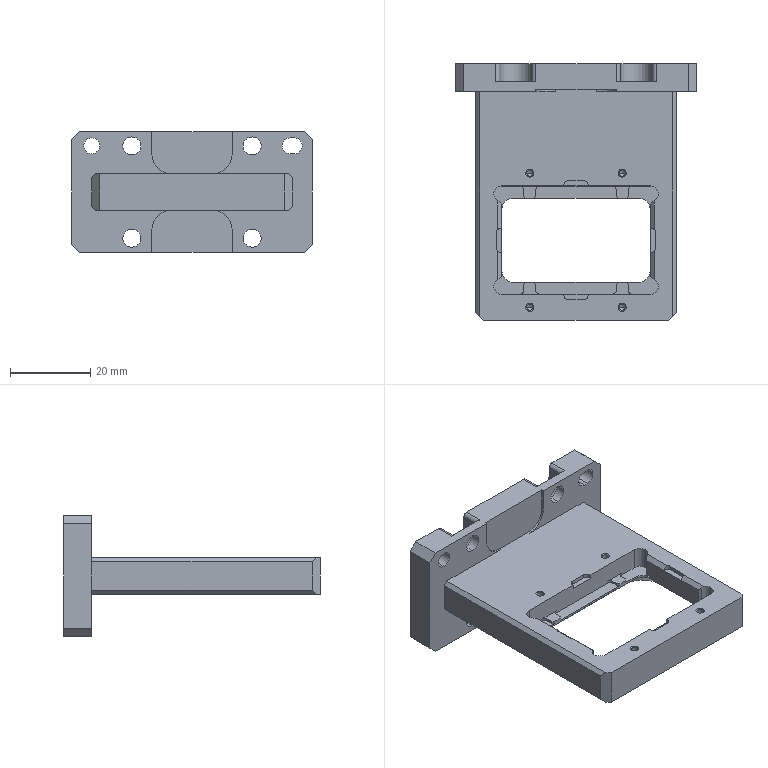NC program | NX | posted with a generic post | part box 60 x 64 x 30 mm
Lines 593 to 2202 of 2202, first 1347 of 1600 lines:
(HOLE_MILLING_COPY , TOOL : D3)
N1184 T03 M6
N1186 G54
N1188 G17 G0 G90 X-25. Y-11.48 B0. C0. S9500 M3
N1190 G43 Z30. H3
N1192 Z0.5
N1194 G94 G3 X-24.8 Y-11.68 R0.2 F1250.
N1196 X-24.6 Y-11.48 R0.2
N1198 X-24.6 Y-11.48 Z0.3 I-0.4 J0.
N1200 X-24.6 Y-11.48 Z0.1 I-0.4 J0.
N1202 X-24.6 Y-11.48 Z-0.1 I-0.4 J0.
N1204 X-24.6 Y-11.48 Z-0.3 I-0.4 J0.
N1206 X-24.6 Y-11.48 Z-0.5 I-0.4 J0.
N1208 X-24.6 Y-11.48 Z-0.7 I-0.4 J0.
N1210 X-24.6 Y-11.48 Z-0.9 I-0.4 J0.
N1212 X-24.6 Y-11.48 Z-1.1 I-0.4 J0.
N1214 X-24.6 Y-11.48 Z-1.3 I-0.4 J0.
N1216 X-24.6 Y-11.48 Z-1.5 I-0.4 J0.
N1218 X-24.6 Y-11.48 Z-1.7 I-0.4 J0.
N1220 X-24.6 Y-11.48 Z-1.9 I-0.4 J0.
N1222 X-24.6 Y-11.48 Z-2.1 I-0.4 J0.
N1224 X-24.6 Y-11.48 Z-2.3 I-0.4 J0.
N1226 X-24.6 Y-11.48 Z-2.5 I-0.4 J0.
N1228 X-24.6 Y-11.48 Z-2.7 I-0.4 J0.
N1230 X-24.6 Y-11.48 Z-2.9 I-0.4 J0.
N1232 X-24.6 Y-11.48 Z-3.1 I-0.4 J0.
N1234 X-24.6 Y-11.48 Z-3.3 I-0.4 J0.
N1236 X-24.6 Y-11.48 Z-3.5 I-0.4 J0.
N1238 X-24.6 Y-11.48 Z-3.7 I-0.4 J0.
N1240 X-24.6 Y-11.48 Z-3.9 I-0.4 J0.
N1242 X-24.6 Y-11.48 Z-4.1 I-0.4 J0.
N1244 X-24.6 Y-11.48 Z-4.3 I-0.4 J0.
N1246 X-24.6 Y-11.48 Z-4.5 I-0.4 J0.
N1248 X-24.6 Y-11.48 Z-4.7 I-0.4 J0.
N1250 X-24.6 Y-11.48 Z-4.9 I-0.4 J0.
N1252 X-24.6 Y-11.48 Z-5.1 I-0.4 J0.
N1254 X-24.6 Y-11.48 Z-5.3 I-0.4 J0.
N1256 X-24.6 Y-11.48 Z-5.5 I-0.4 J0.
N1258 X-24.6 Y-11.48 Z-5.7 I-0.4 J0.
N1260 X-24.6 Y-11.48 Z-5.9 I-0.4 J0.
N1262 X-24.6 Y-11.48 Z-6.1 I-0.4 J0.
N1264 X-24.6 Y-11.48 Z-6.3 I-0.4 J0.
N1266 X-24.6 Y-11.48 Z-6.5 I-0.4 J0.
N1268 X-24.6 Y-11.48 Z-6.7 I-0.4 J0.
N1270 X-24.6 Y-11.48 Z-6.9 I-0.4 J0.
N1272 X-25.4 Y-11.48 Z-7. I-0.4 J0.
N1274 X-25. Y-11.88 R0.4
N1276 X-25.4 Y-11.48 R-0.4
N1278 X-25.2 Y-11.68 R0.2
N1280 X-25. Y-11.48 R0.2
N1282 G0 Z30.
(ZLEVEL_PROFILE_1_1 , TOOL : D3)
N1284 X24.883 Y-11.88
N1286 Z1.
N1288 G1 X25.59 Z0.963 F1000.
N1290 X25.752 Y-11.803 Z0.954
N1292 X25.867 Y-11.664 Z0.944
N1294 X25.91 Y-11.478 Z0.934
N1296 X25.864 Y-11.292 Z0.924
N1298 X25.749 Y-11.154 Z0.915
N1300 X25.59 Y-11.08 Z0.905
N1302 X24.41 Z0.844
N1304 X24.314 Y-11.114 Z0.838
N1306 X24.176 Y-11.229 Z0.829
N1308 X24.1 Y-11.391 Z0.819
N1310 Y-11.57 Z0.81
N1312 X24.177 Y-11.732 Z0.801
N1314 X24.316 Y-11.846 Z0.791
N1316 X24.41 Y-11.88 Z0.786
N1318 X25.59 Z0.724
N1320 X25.752 Y-11.803 Z0.715
N1322 X25.867 Y-11.664 Z0.705
N1324 X25.91 Y-11.478 Z0.695
N1326 X25.864 Y-11.292 Z0.685
N1328 X25.749 Y-11.154 Z0.676
N1330 X25.59 Y-11.08 Z0.667
N1332 X24.41 Z0.605
N1334 X24.314 Y-11.114 Z0.599
N1336 X24.176 Y-11.229 Z0.59
N1338 X24.1 Y-11.391 Z0.581
N1340 Y-11.57 Z0.571
N1342 X24.177 Y-11.732 Z0.562
N1344 X24.316 Y-11.846 Z0.552
N1346 X24.41 Y-11.88 Z0.547
N1348 X25.59 Z0.485
N1350 X25.752 Y-11.803 Z0.476
N1352 X25.867 Y-11.664 Z0.467
N1354 X25.91 Y-11.478 Z0.457
N1356 X25.864 Y-11.292 Z0.446
N1358 X25.749 Y-11.154 Z0.437
N1360 X25.59 Y-11.08 Z0.428
N1362 X24.41 Z0.366
N1364 X24.314 Y-11.114 Z0.361
N1366 X24.176 Y-11.229 Z0.351
N1368 X24.1 Y-11.391 Z0.342
N1370 Y-11.57 Z0.333
N1372 X24.177 Y-11.732 Z0.323
N1374 X24.316 Y-11.846 Z0.314
N1376 X24.41 Y-11.88 Z0.308
N1378 X25.59 Z0.247
N1380 X25.752 Y-11.803 Z0.237
N1382 X25.867 Y-11.664 Z0.228
N1384 X25.91 Y-11.478 Z0.218
N1386 X25.864 Y-11.292 Z0.208
N1388 X25.749 Y-11.154 Z0.198
N1390 X25.59 Y-11.08 Z0.189
N1392 X24.41 Z0.127
N1394 X24.314 Y-11.114 Z0.122
N1396 X24.176 Y-11.229 Z0.113
N1398 X24.1 Y-11.391 Z0.103
N1400 Y-11.57 Z0.094
N1402 X24.177 Y-11.732 Z0.084
N1404 X24.316 Y-11.846 Z0.075
N1406 X24.41 Y-11.88 Z0.07
N1408 X25.59 Z0.008
N1410 X25.752 Y-11.803 Z-0.002
N1412 X25.867 Y-11.664 Z-0.011
N1414 X25.91 Y-11.478 Z-0.021
N1416 X25.864 Y-11.292 Z-0.031
N1418 X25.749 Y-11.154 Z-0.04
N1420 X25.59 Y-11.08 Z-0.05
N1422 X24.41 Z-0.111
N1424 X24.314 Y-11.114 Z-0.117
N1426 X24.176 Y-11.229 Z-0.126
N1428 X24.1 Y-11.391 Z-0.136
N1430 Y-11.57 Z-0.145
N1432 X24.177 Y-11.732 Z-0.154
N1434 X24.316 Y-11.846 Z-0.164
N1436 X24.41 Y-11.88 Z-0.169
N1438 X25. Z-0.2
N1440 X25.5 F1200.
N1442 G3 X25.9 Y-11.48 R0.4
N1444 X25.5 Y-11.08 R0.4
N1446 G1 X24.5
N1448 G3 X24.1 Y-11.48 R0.4
N1450 X24.5 Y-11.88 R0.4
N1452 G1 X25.
N1454 X25.363 Z-0.221
N1456 X25.484 Y-11.874 Z-0.229
N1458 X25.599 Y-11.859 Z-0.235
N1460 X25.652 Y-11.843 Z-0.239
N1462 X25.709 Y-11.812 Z-0.243
N1464 X25.787 Y-11.747 Z-0.249
N1466 X25.818 Y-11.71 Z-0.252
N1468 X25.834 Y-11.686 Z-0.254
N1470 X25.861 Y-11.634 Z-0.257
N1472 X25.887 Y-11.54 Z-0.263
N1474 X25.892 Y-11.493 Z-0.266
N1476 X25.891 Y-11.463 Z-0.268
N1478 X25.884 Y-11.402 Z-0.271
N1480 X25.853 Y-11.31 Z-0.277
N1482 X25.831 Y-11.269 Z-0.28
N1484 X25.812 Y-11.244 Z-0.282
N1486 X25.772 Y-11.197 Z-0.286
N1488 X25.707 Y-11.148 Z-0.291
N1490 X25.673 Y-11.129 Z-0.293
N1492 X25.638 Y-11.112 Z-0.295
N1494 X25.563 Y-11.093 Z-0.3
N1496 X25.443 Y-11.08 Z-0.307
N1498 X25.322 Z-0.314
N1500 X24.597 Z-0.357
N1502 X24.473 Y-11.089 Z-0.364
N1504 X24.412 Y-11.097 Z-0.368
N1506 X24.361 Y-11.113 Z-0.371
N1508 X24.268 Y-11.165 Z-0.378
N1510 X24.204 Y-11.211 Z-0.382
N1512 X24.171 Y-11.253 Z-0.386
N1514 X24.147 Y-11.308 Z-0.389
N1516 X24.126 Y-11.363 Z-0.393
N1518 X24.112 Y-11.421 Z-0.396
N1520 X24.1 Y-11.48 Z-0.4
N1522 G3 X24.5 Y-11.88 R0.4
N1524 G1 X25.
N1526 X25.363 Z-0.421
N1528 X25.484 Y-11.874 Z-0.429
N1530 X25.599 Y-11.859 Z-0.435
N1532 X25.652 Y-11.843 Z-0.439
N1534 X25.709 Y-11.812 Z-0.443
N1536 X25.787 Y-11.747 Z-0.449
N1538 X25.818 Y-11.71 Z-0.452
N1540 X25.834 Y-11.686 Z-0.454
N1542 X25.861 Y-11.634 Z-0.457
N1544 X25.887 Y-11.54 Z-0.463
N1546 X25.892 Y-11.493 Z-0.466
N1548 X25.891 Y-11.463 Z-0.468
N1550 X25.884 Y-11.402 Z-0.471
N1552 X25.853 Y-11.31 Z-0.477
N1554 X25.831 Y-11.269 Z-0.48
N1556 X25.812 Y-11.244 Z-0.482
N1558 X25.771 Y-11.197 Z-0.486
N1560 X25.707 Y-11.148 Z-0.491
N1562 X25.673 Y-11.129 Z-0.493
N1564 X25.638 Y-11.112 Z-0.495
N1566 X25.563 Y-11.093 Z-0.5
N1568 X25.443 Y-11.08 Z-0.507
N1570 X25.322 Z-0.514
N1572 X24.597 Z-0.557
N1574 X24.473 Y-11.089 Z-0.564
N1576 X24.412 Y-11.097 Z-0.568
N1578 X24.361 Y-11.113 Z-0.571
N1580 X24.268 Y-11.165 Z-0.578
N1582 X24.204 Y-11.211 Z-0.582
N1584 X24.171 Y-11.253 Z-0.586
N1586 X24.147 Y-11.308 Z-0.589
N1588 X24.126 Y-11.363 Z-0.593
N1590 X24.112 Y-11.421 Z-0.596
N1592 X24.1 Y-11.48 Z-0.6
N1594 G3 X24.5 Y-11.88 R0.4
N1596 G1 X25.
N1598 X25.363 Z-0.621
N1600 X25.484 Y-11.874 Z-0.629
N1602 X25.599 Y-11.859 Z-0.635
N1604 X25.652 Y-11.843 Z-0.639
N1606 X25.709 Y-11.811 Z-0.643
N1608 X25.787 Y-11.747 Z-0.649
N1610 X25.818 Y-11.71 Z-0.652
N1612 X25.834 Y-11.686 Z-0.654
N1614 X25.861 Y-11.634 Z-0.657
N1616 X25.887 Y-11.54 Z-0.663
N1618 X25.892 Y-11.493 Z-0.666
N1620 X25.891 Y-11.463 Z-0.668
N1622 X25.884 Y-11.402 Z-0.671
N1624 X25.853 Y-11.31 Z-0.677
N1626 X25.831 Y-11.269 Z-0.68
N1628 X25.812 Y-11.244 Z-0.682
N1630 X25.771 Y-11.197 Z-0.686
N1632 X25.707 Y-11.148 Z-0.691
N1634 X25.673 Y-11.129 Z-0.693
N1636 X25.638 Y-11.112 Z-0.695
N1638 X25.563 Y-11.093 Z-0.7
N1640 X25.443 Y-11.08 Z-0.707
N1642 X25.322 Z-0.714
N1644 X24.597 Z-0.757
N1646 X24.473 Y-11.089 Z-0.764
N1648 X24.412 Y-11.097 Z-0.768
N1650 X24.361 Y-11.113 Z-0.771
N1652 X24.268 Y-11.165 Z-0.778
N1654 X24.204 Y-11.211 Z-0.782
N1656 X24.171 Y-11.253 Z-0.786
N1658 X24.147 Y-11.308 Z-0.789
N1660 X24.126 Y-11.363 Z-0.793
N1662 X24.112 Y-11.421 Z-0.796
N1664 X24.1 Y-11.48 Z-0.8
N1666 G3 X24.5 Y-11.88 R0.4
N1668 G1 X25.
N1670 X25.363 Z-0.821
N1672 X25.484 Y-11.874 Z-0.829
N1674 X25.599 Y-11.859 Z-0.835
N1676 X25.652 Y-11.843 Z-0.839
N1678 X25.709 Y-11.811 Z-0.843
N1680 X25.787 Y-11.747 Z-0.849
N1682 X25.818 Y-11.71 Z-0.852
N1684 X25.834 Y-11.686 Z-0.854
N1686 X25.861 Y-11.634 Z-0.857
N1688 X25.887 Y-11.54 Z-0.863
N1690 X25.892 Y-11.493 Z-0.866
N1692 X25.891 Y-11.463 Z-0.868
N1694 X25.884 Y-11.402 Z-0.871
N1696 X25.853 Y-11.31 Z-0.877
N1698 X25.831 Y-11.269 Z-0.88
N1700 X25.812 Y-11.244 Z-0.882
N1702 X25.771 Y-11.197 Z-0.886
N1704 X25.707 Y-11.148 Z-0.891
N1706 X25.673 Y-11.129 Z-0.893
N1708 X25.638 Y-11.112 Z-0.895
N1710 X25.563 Y-11.093 Z-0.9
N1712 X25.443 Y-11.08 Z-0.907
N1714 X25.322 Z-0.914
N1716 X24.597 Z-0.957
N1718 X24.473 Y-11.089 Z-0.964
N1720 X24.412 Y-11.097 Z-0.968
N1722 X24.361 Y-11.113 Z-0.971
N1724 X24.268 Y-11.165 Z-0.978
N1726 X24.204 Y-11.211 Z-0.982
N1728 X24.171 Y-11.253 Z-0.986
N1730 X24.147 Y-11.308 Z-0.989
N1732 X24.126 Y-11.363 Z-0.993
N1734 X24.112 Y-11.421 Z-0.996
N1736 X24.1 Y-11.48 Z-1.
N1738 G3 X24.5 Y-11.88 R0.4
N1740 G1 X25.
N1742 X25.363 Z-1.021
N1744 X25.484 Y-11.874 Z-1.029
N1746 X25.599 Y-11.859 Z-1.035
N1748 X25.653 Y-11.843 Z-1.039
N1750 X25.709 Y-11.811 Z-1.043
N1752 X25.787 Y-11.747 Z-1.049
N1754 X25.818 Y-11.71 Z-1.052
N1756 X25.834 Y-11.686 Z-1.054
N1758 X25.861 Y-11.634 Z-1.057
N1760 X25.887 Y-11.54 Z-1.063
N1762 X25.892 Y-11.493 Z-1.066
N1764 X25.891 Y-11.463 Z-1.068
N1766 X25.884 Y-11.402 Z-1.071
N1768 X25.853 Y-11.31 Z-1.077
N1770 X25.831 Y-11.269 Z-1.08
N1772 X25.812 Y-11.244 Z-1.082
N1774 X25.771 Y-11.197 Z-1.086
N1776 X25.707 Y-11.148 Z-1.091
N1778 X25.673 Y-11.129 Z-1.093
N1780 X25.638 Y-11.112 Z-1.095
N1782 X25.563 Y-11.093 Z-1.1
N1784 X25.443 Y-11.08 Z-1.107
N1786 X25.322 Z-1.114
N1788 X24.597 Z-1.157
N1790 X24.473 Y-11.089 Z-1.164
N1792 X24.412 Y-11.097 Z-1.168
N1794 X24.361 Y-11.113 Z-1.171
N1796 X24.268 Y-11.165 Z-1.178
N1798 X24.204 Y-11.211 Z-1.182
N1800 X24.171 Y-11.253 Z-1.186
N1802 X24.147 Y-11.308 Z-1.189
N1804 X24.126 Y-11.363 Z-1.193
N1806 X24.112 Y-11.421 Z-1.196
N1808 X24.1 Y-11.48 Z-1.2
N1810 G3 X24.5 Y-11.88 R0.4
N1812 G1 X25.
N1814 X25.363 Z-1.221
N1816 X25.484 Y-11.874 Z-1.229
N1818 X25.599 Y-11.859 Z-1.235
N1820 X25.653 Y-11.843 Z-1.239
N1822 X25.709 Y-11.811 Z-1.243
N1824 X25.787 Y-11.747 Z-1.249
N1826 X25.818 Y-11.71 Z-1.252
N1828 X25.834 Y-11.686 Z-1.254
N1830 X25.861 Y-11.634 Z-1.257
N1832 X25.887 Y-11.54 Z-1.263
N1834 X25.892 Y-11.493 Z-1.266
N1836 X25.891 Y-11.463 Z-1.268
N1838 X25.884 Y-11.402 Z-1.271
N1840 X25.853 Y-11.31 Z-1.277
N1842 X25.831 Y-11.269 Z-1.28
N1844 X25.812 Y-11.244 Z-1.282
N1846 X25.771 Y-11.197 Z-1.286
N1848 X25.707 Y-11.148 Z-1.291
N1850 X25.673 Y-11.129 Z-1.293
N1852 X25.638 Y-11.112 Z-1.295
N1854 X25.563 Y-11.093 Z-1.3
N1856 X25.443 Y-11.08 Z-1.307
N1858 X25.322 Z-1.314
N1860 X24.597 Z-1.357
N1862 X24.473 Y-11.089 Z-1.364
N1864 X24.412 Y-11.097 Z-1.368
N1866 X24.361 Y-11.113 Z-1.371
N1868 X24.268 Y-11.165 Z-1.378
N1870 X24.204 Y-11.211 Z-1.382
N1872 X24.171 Y-11.253 Z-1.386
N1874 X24.147 Y-11.308 Z-1.389
N1876 X24.126 Y-11.363 Z-1.393
N1878 X24.112 Y-11.421 Z-1.396
N1880 X24.1 Y-11.48 Z-1.4
N1882 G3 X24.5 Y-11.88 R0.4
N1884 G1 X25.
N1886 X25.363 Z-1.421
N1888 X25.484 Y-11.874 Z-1.429
N1890 X25.599 Y-11.859 Z-1.435
N1892 X25.653 Y-11.843 Z-1.439
N1894 X25.709 Y-11.811 Z-1.443
N1896 X25.787 Y-11.747 Z-1.449
N1898 X25.818 Y-11.71 Z-1.452
N1900 X25.834 Y-11.686 Z-1.454
N1902 X25.861 Y-11.634 Z-1.457
N1904 X25.887 Y-11.54 Z-1.463
N1906 X25.892 Y-11.493 Z-1.466
N1908 X25.891 Y-11.463 Z-1.468
N1910 X25.884 Y-11.402 Z-1.471
N1912 X25.853 Y-11.31 Z-1.477
N1914 X25.831 Y-11.269 Z-1.48
N1916 X25.812 Y-11.244 Z-1.482
N1918 X25.771 Y-11.197 Z-1.486
N1920 X25.707 Y-11.148 Z-1.491
N1922 X25.673 Y-11.129 Z-1.493
N1924 X25.638 Y-11.112 Z-1.495
N1926 X25.563 Y-11.093 Z-1.5
N1928 X25.443 Y-11.08 Z-1.507
N1930 X25.322 Z-1.514
N1932 X24.597 Z-1.557
N1934 X24.473 Y-11.089 Z-1.564
N1936 X24.412 Y-11.097 Z-1.568
N1938 X24.361 Y-11.113 Z-1.571
N1940 X24.268 Y-11.165 Z-1.578
N1942 X24.204 Y-11.211 Z-1.582
N1944 X24.171 Y-11.253 Z-1.586
N1946 X24.147 Y-11.308 Z-1.589
N1948 X24.126 Y-11.363 Z-1.593
N1950 X24.112 Y-11.421 Z-1.596
N1952 X24.1 Y-11.48 Z-1.6
N1954 G3 X24.5 Y-11.88 R0.4
N1956 G1 X25.
N1958 X25.363 Z-1.621
N1960 X25.484 Y-11.874 Z-1.629
N1962 X25.599 Y-11.859 Z-1.635
N1964 X25.653 Y-11.843 Z-1.639
N1966 X25.709 Y-11.811 Z-1.643
N1968 X25.787 Y-11.747 Z-1.649
N1970 X25.818 Y-11.71 Z-1.652
N1972 X25.834 Y-11.686 Z-1.654
N1974 X25.861 Y-11.634 Z-1.657
N1976 X25.887 Y-11.54 Z-1.663
N1978 X25.892 Y-11.493 Z-1.666
N1980 X25.891 Y-11.463 Z-1.668
N1982 X25.884 Y-11.402 Z-1.671
N1984 X25.853 Y-11.31 Z-1.677
N1986 X25.831 Y-11.269 Z-1.68
N1988 X25.812 Y-11.244 Z-1.682
N1990 X25.771 Y-11.197 Z-1.686
N1992 X25.707 Y-11.148 Z-1.691
N1994 X25.673 Y-11.129 Z-1.693
N1996 X25.638 Y-11.112 Z-1.695
N1998 X25.563 Y-11.093 Z-1.7
N2000 X25.443 Y-11.08 Z-1.707
N2002 X25.322 Z-1.714
N2004 X24.597 Z-1.757
N2006 X24.473 Y-11.089 Z-1.764
N2008 X24.412 Y-11.097 Z-1.768
N2010 X24.361 Y-11.113 Z-1.771
N2012 X24.268 Y-11.165 Z-1.778
N2014 X24.204 Y-11.211 Z-1.782
N2016 X24.171 Y-11.253 Z-1.786
N2018 X24.147 Y-11.308 Z-1.789
N2020 X24.126 Y-11.363 Z-1.793
N2022 X24.112 Y-11.421 Z-1.796
N2024 X24.1 Y-11.48 Z-1.8
N2026 G3 X24.5 Y-11.88 R0.4
N2028 G1 X25.
N2030 X25.363 Z-1.821
N2032 X25.484 Y-11.874 Z-1.829
N2034 X25.599 Y-11.859 Z-1.835
N2036 X25.653 Y-11.843 Z-1.839
N2038 X25.709 Y-11.811 Z-1.843
N2040 X25.787 Y-11.747 Z-1.849
N2042 X25.818 Y-11.71 Z-1.852
N2044 X25.834 Y-11.686 Z-1.854
N2046 X25.861 Y-11.634 Z-1.857
N2048 X25.887 Y-11.54 Z-1.863
N2050 X25.892 Y-11.493 Z-1.866
N2052 X25.891 Y-11.463 Z-1.868
N2054 X25.884 Y-11.402 Z-1.871
N2056 X25.853 Y-11.31 Z-1.877
N2058 X25.831 Y-11.269 Z-1.88
N2060 X25.812 Y-11.244 Z-1.882
N2062 X25.771 Y-11.197 Z-1.886
N2064 X25.707 Y-11.148 Z-1.891
N2066 X25.673 Y-11.129 Z-1.893
N2068 X25.638 Y-11.112 Z-1.895
N2070 X25.563 Y-11.093 Z-1.9
N2072 X25.443 Y-11.08 Z-1.907
N2074 X25.322 Z-1.914
N2076 X24.597 Z-1.957
N2078 X24.473 Y-11.089 Z-1.964
N2080 X24.412 Y-11.097 Z-1.968
N2082 X24.361 Y-11.113 Z-1.971
N2084 X24.268 Y-11.165 Z-1.978
N2086 X24.204 Y-11.211 Z-1.982
N2088 X24.171 Y-11.253 Z-1.986
N2090 X24.147 Y-11.308 Z-1.989
N2092 X24.126 Y-11.363 Z-1.993
N2094 X24.112 Y-11.421 Z-1.996
N2096 X24.1 Y-11.48 Z-2.
N2098 G3 X24.5 Y-11.88 R0.4
N2100 G1 X25.
N2102 X25.363 Z-2.021
N2104 X25.484 Y-11.874 Z-2.029
N2106 X25.599 Y-11.859 Z-2.035
N2108 X25.653 Y-11.843 Z-2.039
N2110 X25.709 Y-11.811 Z-2.043
N2112 X25.787 Y-11.747 Z-2.049
N2114 X25.818 Y-11.71 Z-2.052
N2116 X25.834 Y-11.686 Z-2.054
N2118 X25.861 Y-11.634 Z-2.057
N2120 X25.887 Y-11.54 Z-2.063
N2122 X25.892 Y-11.493 Z-2.066
N2124 X25.891 Y-11.463 Z-2.068
N2126 X25.884 Y-11.402 Z-2.071
N2128 X25.853 Y-11.31 Z-2.077
N2130 X25.831 Y-11.269 Z-2.08
N2132 X25.812 Y-11.244 Z-2.082
N2134 X25.771 Y-11.197 Z-2.086
N2136 X25.707 Y-11.148 Z-2.091
N2138 X25.673 Y-11.129 Z-2.093
N2140 X25.638 Y-11.112 Z-2.095
N2142 X25.563 Y-11.093 Z-2.1
N2144 X25.443 Y-11.08 Z-2.107
N2146 X25.322 Z-2.114
N2148 X24.597 Z-2.157
N2150 X24.473 Y-11.089 Z-2.164
N2152 X24.412 Y-11.097 Z-2.168
N2154 X24.361 Y-11.113 Z-2.171
N2156 X24.268 Y-11.165 Z-2.178
N2158 X24.204 Y-11.211 Z-2.182
N2160 X24.171 Y-11.253 Z-2.186
N2162 X24.147 Y-11.308 Z-2.189
N2164 X24.126 Y-11.363 Z-2.193
N2166 X24.112 Y-11.421 Z-2.196
N2168 X24.1 Y-11.48 Z-2.2
N2170 G3 X24.5 Y-11.88 R0.4
N2172 G1 X25.
N2174 X25.363 Z-2.221
N2176 X25.484 Y-11.874 Z-2.229
N2178 X25.599 Y-11.859 Z-2.235
N2180 X25.653 Y-11.843 Z-2.239
N2182 X25.709 Y-11.811 Z-2.243
N2184 X25.787 Y-11.747 Z-2.249
N2186 X25.818 Y-11.71 Z-2.252
N2188 X25.834 Y-11.686 Z-2.254
N2190 X25.861 Y-11.634 Z-2.257
N2192 X25.887 Y-11.54 Z-2.263
N2194 X25.892 Y-11.493 Z-2.266
N2196 X25.891 Y-11.463 Z-2.268
N2198 X25.884 Y-11.402 Z-2.271
N2200 X25.853 Y-11.31 Z-2.277
N2202 X25.831 Y-11.269 Z-2.28
N2204 X25.812 Y-11.244 Z-2.282
N2206 X25.771 Y-11.197 Z-2.286
N2208 X25.707 Y-11.148 Z-2.291
N2210 X25.673 Y-11.129 Z-2.293
N2212 X25.638 Y-11.112 Z-2.295
N2214 X25.563 Y-11.093 Z-2.3
N2216 X25.443 Y-11.08 Z-2.307
N2218 X25.322 Z-2.314
N2220 X24.597 Z-2.357
N2222 X24.473 Y-11.089 Z-2.364
N2224 X24.412 Y-11.097 Z-2.368
N2226 X24.361 Y-11.113 Z-2.371
N2228 X24.268 Y-11.165 Z-2.378
N2230 X24.204 Y-11.211 Z-2.382
N2232 X24.171 Y-11.253 Z-2.386
N2234 X24.147 Y-11.308 Z-2.389
N2236 X24.126 Y-11.363 Z-2.393
N2238 X24.112 Y-11.421 Z-2.396
N2240 X24.1 Y-11.48 Z-2.4
N2242 G3 X24.5 Y-11.88 R0.4
N2244 G1 X25.
N2246 X25.363 Z-2.421
N2248 X25.484 Y-11.874 Z-2.429
N2250 X25.599 Y-11.859 Z-2.435
N2252 X25.653 Y-11.843 Z-2.439
N2254 X25.709 Y-11.811 Z-2.443
N2256 X25.787 Y-11.747 Z-2.449
N2258 X25.818 Y-11.71 Z-2.452
N2260 X25.834 Y-11.686 Z-2.454
N2262 X25.861 Y-11.634 Z-2.457
N2264 X25.887 Y-11.54 Z-2.463
N2266 X25.892 Y-11.493 Z-2.466
N2268 X25.891 Y-11.463 Z-2.468
N2270 X25.884 Y-11.402 Z-2.471
N2272 X25.853 Y-11.31 Z-2.477
N2274 X25.831 Y-11.269 Z-2.48
N2276 X25.812 Y-11.244 Z-2.482
N2278 X25.771 Y-11.197 Z-2.486
N2280 X25.707 Y-11.148 Z-2.491
N2282 X25.673 Y-11.129 Z-2.493
N2284 X25.638 Y-11.112 Z-2.495
N2286 X25.563 Y-11.093 Z-2.5
N2288 X25.443 Y-11.08 Z-2.507
N2290 X25.322 Z-2.514
N2292 X24.597 Z-2.557
N2294 X24.473 Y-11.089 Z-2.564
N2296 X24.412 Y-11.097 Z-2.568
N2298 X24.361 Y-11.113 Z-2.571
N2300 X24.268 Y-11.165 Z-2.578
N2302 X24.204 Y-11.211 Z-2.582
N2304 X24.171 Y-11.253 Z-2.586
N2306 X24.147 Y-11.308 Z-2.589
N2308 X24.126 Y-11.363 Z-2.593
N2310 X24.112 Y-11.421 Z-2.596
N2312 X24.1 Y-11.48 Z-2.6
N2314 G3 X24.5 Y-11.88 R0.4
N2316 G1 X25.
N2318 X25.363 Z-2.621
N2320 X25.484 Y-11.874 Z-2.629
N2322 X25.599 Y-11.859 Z-2.635
N2324 X25.653 Y-11.843 Z-2.639
N2326 X25.709 Y-11.811 Z-2.643
N2328 X25.787 Y-11.747 Z-2.649
N2330 X25.818 Y-11.71 Z-2.652
N2332 X25.834 Y-11.686 Z-2.654
N2334 X25.861 Y-11.634 Z-2.657
N2336 X25.887 Y-11.54 Z-2.663
N2338 X25.892 Y-11.493 Z-2.666
N2340 X25.891 Y-11.463 Z-2.668
N2342 X25.884 Y-11.402 Z-2.671
N2344 X25.853 Y-11.31 Z-2.677
N2346 X25.831 Y-11.269 Z-2.68
N2348 X25.812 Y-11.244 Z-2.682
N2350 X25.771 Y-11.197 Z-2.686
N2352 X25.707 Y-11.148 Z-2.691
N2354 X25.673 Y-11.129 Z-2.693
N2356 X25.638 Y-11.112 Z-2.695
N2358 X25.563 Y-11.093 Z-2.7
N2360 X25.443 Y-11.08 Z-2.707
N2362 X25.322 Z-2.714
N2364 X24.597 Z-2.757
N2366 X24.473 Y-11.089 Z-2.764
N2368 X24.412 Y-11.097 Z-2.768
N2370 X24.361 Y-11.113 Z-2.771
N2372 X24.268 Y-11.165 Z-2.778
N2374 X24.204 Y-11.211 Z-2.782
N2376 X24.171 Y-11.253 Z-2.786
N2378 X24.147 Y-11.308 Z-2.789
N2380 X24.126 Y-11.363 Z-2.793
N2382 X24.112 Y-11.421 Z-2.796
N2384 X24.1 Y-11.48 Z-2.8
N2386 G3 X24.5 Y-11.88 R0.4
N2388 G1 X25.
N2390 X25.363 Z-2.821
N2392 X25.484 Y-11.874 Z-2.829
N2394 X25.599 Y-11.859 Z-2.835
N2396 X25.653 Y-11.843 Z-2.839
N2398 X25.709 Y-11.811 Z-2.843
N2400 X25.787 Y-11.747 Z-2.849
N2402 X25.818 Y-11.71 Z-2.852
N2404 X25.834 Y-11.686 Z-2.854
N2406 X25.861 Y-11.634 Z-2.857
N2408 X25.887 Y-11.54 Z-2.863
N2410 X25.892 Y-11.493 Z-2.866
N2412 X25.891 Y-11.463 Z-2.868
N2414 X25.884 Y-11.402 Z-2.871
N2416 X25.853 Y-11.31 Z-2.877
N2418 X25.831 Y-11.269 Z-2.88
N2420 X25.812 Y-11.244 Z-2.882
N2422 X25.771 Y-11.197 Z-2.886
N2424 X25.707 Y-11.148 Z-2.891
N2426 X25.673 Y-11.129 Z-2.893
N2428 X25.638 Y-11.112 Z-2.895
N2430 X25.563 Y-11.093 Z-2.9
N2432 X25.443 Y-11.08 Z-2.907
N2434 X25.322 Z-2.914
N2436 X24.597 Z-2.957
N2438 X24.473 Y-11.089 Z-2.964
N2440 X24.412 Y-11.097 Z-2.968
N2442 X24.361 Y-11.113 Z-2.971
N2444 X24.268 Y-11.165 Z-2.978
N2446 X24.204 Y-11.211 Z-2.982
N2448 X24.171 Y-11.253 Z-2.986
N2450 X24.147 Y-11.308 Z-2.989
N2452 X24.126 Y-11.363 Z-2.993
N2454 X24.112 Y-11.421 Z-2.996
N2456 X24.1 Y-11.48 Z-3.
N2458 G3 X24.5 Y-11.88 R0.4
N2460 G1 X25.
N2462 X25.363 Z-3.021
N2464 X25.484 Y-11.874 Z-3.029
N2466 X25.599 Y-11.859 Z-3.035
N2468 X25.653 Y-11.843 Z-3.039
N2470 X25.709 Y-11.811 Z-3.043
N2472 X25.787 Y-11.747 Z-3.049
N2474 X25.818 Y-11.71 Z-3.052
N2476 X25.834 Y-11.686 Z-3.054
N2478 X25.861 Y-11.634 Z-3.057
N2480 X25.887 Y-11.54 Z-3.063
N2482 X25.892 Y-11.493 Z-3.066
N2484 X25.891 Y-11.463 Z-3.068
N2486 X25.884 Y-11.402 Z-3.071
N2488 X25.853 Y-11.31 Z-3.077
N2490 X25.831 Y-11.269 Z-3.08
N2492 X25.812 Y-11.244 Z-3.082
N2494 X25.771 Y-11.197 Z-3.086
N2496 X25.707 Y-11.148 Z-3.091
N2498 X25.673 Y-11.129 Z-3.093
N2500 X25.638 Y-11.112 Z-3.095
N2502 X25.563 Y-11.093 Z-3.1
N2504 X25.443 Y-11.08 Z-3.107
N2506 X25.322 Z-3.114
N2508 X24.597 Z-3.157
N2510 X24.473 Y-11.089 Z-3.164
N2512 X24.412 Y-11.097 Z-3.168
N2514 X24.361 Y-11.113 Z-3.171
N2516 X24.268 Y-11.165 Z-3.178
N2518 X24.204 Y-11.211 Z-3.182
N2520 X24.171 Y-11.253 Z-3.186
N2522 X24.147 Y-11.308 Z-3.189
N2524 X24.126 Y-11.363 Z-3.193
N2526 X24.112 Y-11.421 Z-3.196
N2528 X24.1 Y-11.48 Z-3.2
N2530 G3 X24.5 Y-11.88 R0.4
N2532 G1 X25.
N2534 X25.363 Z-3.221
N2536 X25.484 Y-11.874 Z-3.229
N2538 X25.599 Y-11.859 Z-3.235
N2540 X25.653 Y-11.842 Z-3.239
N2542 X25.709 Y-11.811 Z-3.243
N2544 X25.787 Y-11.747 Z-3.249
N2546 X25.818 Y-11.71 Z-3.252
N2548 X25.834 Y-11.686 Z-3.254
N2550 X25.861 Y-11.634 Z-3.257
N2552 X25.887 Y-11.54 Z-3.263
N2554 X25.892 Y-11.493 Z-3.266
N2556 X25.891 Y-11.463 Z-3.268
N2558 X25.884 Y-11.402 Z-3.271
N2560 X25.853 Y-11.31 Z-3.277
N2562 X25.831 Y-11.269 Z-3.28
N2564 X25.812 Y-11.244 Z-3.282
N2566 X25.771 Y-11.197 Z-3.286
N2568 X25.707 Y-11.148 Z-3.291
N2570 X25.673 Y-11.129 Z-3.293
N2572 X25.638 Y-11.112 Z-3.295
N2574 X25.563 Y-11.093 Z-3.3
N2576 X25.443 Y-11.08 Z-3.307
N2578 X25.322 Z-3.314
N2580 X24.597 Z-3.357
N2582 X24.473 Y-11.089 Z-3.364
N2584 X24.412 Y-11.097 Z-3.368
N2586 X24.361 Y-11.113 Z-3.371
N2588 X24.268 Y-11.165 Z-3.378
N2590 X24.204 Y-11.211 Z-3.382
N2592 X24.171 Y-11.253 Z-3.386
N2594 X24.147 Y-11.308 Z-3.389
N2596 X24.126 Y-11.363 Z-3.393
N2598 X24.112 Y-11.421 Z-3.396
N2600 X24.1 Y-11.48 Z-3.4
N2602 G3 X24.5 Y-11.88 R0.4
N2604 G1 X25.
N2606 X25.363 Z-3.421
N2608 X25.484 Y-11.874 Z-3.429
N2610 X25.599 Y-11.859 Z-3.435
N2612 X25.653 Y-11.842 Z-3.439
N2614 X25.709 Y-11.811 Z-3.443
N2616 X25.787 Y-11.747 Z-3.449
N2618 X25.818 Y-11.71 Z-3.452
N2620 X25.834 Y-11.686 Z-3.454
N2622 X25.861 Y-11.634 Z-3.457
N2624 X25.887 Y-11.54 Z-3.463
N2626 X25.892 Y-11.493 Z-3.466
N2628 X25.891 Y-11.463 Z-3.468
N2630 X25.884 Y-11.402 Z-3.471
N2632 X25.853 Y-11.31 Z-3.477
N2634 X25.831 Y-11.269 Z-3.48
N2636 X25.812 Y-11.244 Z-3.482
N2638 X25.771 Y-11.197 Z-3.486
N2640 X25.707 Y-11.148 Z-3.491
N2642 X25.673 Y-11.129 Z-3.493
N2644 X25.638 Y-11.112 Z-3.495
N2646 X25.563 Y-11.093 Z-3.5
N2648 X25.443 Y-11.08 Z-3.507
N2650 X25.322 Z-3.514
N2652 X24.597 Z-3.557
N2654 X24.473 Y-11.089 Z-3.564
N2656 X24.412 Y-11.097 Z-3.568
N2658 X24.361 Y-11.113 Z-3.571
N2660 X24.268 Y-11.165 Z-3.578
N2662 X24.204 Y-11.211 Z-3.582
N2664 X24.171 Y-11.253 Z-3.586
N2666 X24.147 Y-11.308 Z-3.589
N2668 X24.126 Y-11.363 Z-3.593
N2670 X24.112 Y-11.421 Z-3.596
N2672 X24.1 Y-11.48 Z-3.6
N2674 G3 X24.5 Y-11.88 R0.4
N2676 G1 X25.
N2678 X25.363 Z-3.621
N2680 X25.484 Y-11.874 Z-3.629
N2682 X25.599 Y-11.859 Z-3.635
N2684 X25.653 Y-11.842 Z-3.639
N2686 X25.709 Y-11.811 Z-3.643
N2688 X25.787 Y-11.747 Z-3.649
N2690 X25.818 Y-11.71 Z-3.652
N2692 X25.834 Y-11.686 Z-3.654
N2694 X25.861 Y-11.634 Z-3.657
N2696 X25.887 Y-11.54 Z-3.663
N2698 X25.892 Y-11.493 Z-3.666
N2700 X25.891 Y-11.463 Z-3.668
N2702 X25.884 Y-11.402 Z-3.671
N2704 X25.853 Y-11.31 Z-3.677
N2706 X25.831 Y-11.269 Z-3.68
N2708 X25.812 Y-11.244 Z-3.682
N2710 X25.771 Y-11.197 Z-3.686
N2712 X25.707 Y-11.148 Z-3.691
N2714 X25.673 Y-11.129 Z-3.693
N2716 X25.638 Y-11.112 Z-3.695
N2718 X25.563 Y-11.093 Z-3.7
N2720 X25.443 Y-11.08 Z-3.707
N2722 X25.322 Z-3.714
N2724 X24.597 Z-3.757
N2726 X24.473 Y-11.089 Z-3.764
N2728 X24.412 Y-11.097 Z-3.768
N2730 X24.361 Y-11.113 Z-3.771
N2732 X24.268 Y-11.165 Z-3.778
N2734 X24.204 Y-11.211 Z-3.782
N2736 X24.171 Y-11.253 Z-3.786
N2738 X24.147 Y-11.308 Z-3.789
N2740 X24.126 Y-11.363 Z-3.793
N2742 X24.112 Y-11.421 Z-3.796
N2744 X24.1 Y-11.48 Z-3.8
N2746 G3 X24.5 Y-11.88 R0.4
N2748 G1 X25.
N2750 X25.363 Z-3.821
N2752 X25.484 Y-11.874 Z-3.829
N2754 X25.599 Y-11.859 Z-3.835
N2756 X25.653 Y-11.842 Z-3.839
N2758 X25.709 Y-11.811 Z-3.843
N2760 X25.787 Y-11.747 Z-3.849
N2762 X25.818 Y-11.71 Z-3.852
N2764 X25.834 Y-11.686 Z-3.854
N2766 X25.861 Y-11.634 Z-3.857
N2768 X25.887 Y-11.54 Z-3.863
N2770 X25.892 Y-11.493 Z-3.866
N2772 X25.891 Y-11.463 Z-3.868
N2774 X25.884 Y-11.402 Z-3.871
N2776 X25.853 Y-11.31 Z-3.877
N2778 X25.831 Y-11.269 Z-3.88
N2780 X25.812 Y-11.244 Z-3.882
N2782 X25.771 Y-11.197 Z-3.886
N2784 X25.707 Y-11.148 Z-3.891
N2786 X25.673 Y-11.129 Z-3.893
N2788 X25.638 Y-11.112 Z-3.895
N2790 X25.563 Y-11.093 Z-3.9
N2792 X25.443 Y-11.08 Z-3.907
N2794 X25.322 Z-3.914
N2796 X24.597 Z-3.957
N2798 X24.473 Y-11.089 Z-3.964
N2800 X24.412 Y-11.097 Z-3.968
N2802 X24.361 Y-11.113 Z-3.971
N2804 X24.268 Y-11.165 Z-3.978
N2806 X24.204 Y-11.211 Z-3.982
N2808 X24.171 Y-11.253 Z-3.986
N2810 X24.147 Y-11.308 Z-3.989
N2812 X24.126 Y-11.363 Z-3.993
N2814 X24.112 Y-11.421 Z-3.996
N2816 X24.1 Y-11.48 Z-4.
N2818 G3 X24.5 Y-11.88 R0.4
N2820 G1 X25.
N2822 X25.363 Z-4.021
N2824 X25.484 Y-11.874 Z-4.029
N2826 X25.599 Y-11.859 Z-4.035
N2828 X25.653 Y-11.842 Z-4.039
N2830 X25.709 Y-11.811 Z-4.043
N2832 X25.787 Y-11.747 Z-4.049
N2834 X25.818 Y-11.71 Z-4.052
N2836 X25.834 Y-11.686 Z-4.054
N2838 X25.861 Y-11.634 Z-4.057
N2840 X25.887 Y-11.54 Z-4.063
N2842 X25.892 Y-11.493 Z-4.066
N2844 X25.891 Y-11.463 Z-4.068
N2846 X25.884 Y-11.402 Z-4.071
N2848 X25.853 Y-11.31 Z-4.077
N2850 X25.831 Y-11.269 Z-4.08
N2852 X25.812 Y-11.244 Z-4.082
N2854 X25.771 Y-11.197 Z-4.086
N2856 X25.707 Y-11.148 Z-4.091
N2858 X25.673 Y-11.129 Z-4.093
N2860 X25.638 Y-11.112 Z-4.095
N2862 X25.563 Y-11.093 Z-4.1
N2864 X25.443 Y-11.08 Z-4.107
N2866 X25.322 Z-4.114
N2868 X24.597 Z-4.157
N2870 X24.473 Y-11.089 Z-4.164
N2872 X24.412 Y-11.097 Z-4.168
N2874 X24.361 Y-11.113 Z-4.171
N2876 X24.268 Y-11.165 Z-4.178
N2878 X24.204 Y-11.211 Z-4.182
N2880 X24.171 Y-11.253 Z-4.186
N2882 X24.147 Y-11.308 Z-4.189
N2884 X24.126 Y-11.363 Z-4.193
N2886 X24.112 Y-11.421 Z-4.196
N2888 X24.1 Y-11.48 Z-4.2
N2890 G3 X24.5 Y-11.88 R0.4
N2892 G1 X25.
N2894 X25.363 Z-4.221
N2896 X25.484 Y-11.874 Z-4.229
N2898 X25.599 Y-11.859 Z-4.235
N2900 X25.653 Y-11.842 Z-4.239
N2902 X25.709 Y-11.811 Z-4.243
N2904 X25.787 Y-11.747 Z-4.249
N2906 X25.818 Y-11.71 Z-4.252
N2908 X25.834 Y-11.686 Z-4.254
N2910 X25.861 Y-11.634 Z-4.257
N2912 X25.887 Y-11.54 Z-4.263
N2914 X25.892 Y-11.493 Z-4.266
N2916 X25.891 Y-11.463 Z-4.268
N2918 X25.884 Y-11.402 Z-4.271
N2920 X25.853 Y-11.31 Z-4.277
N2922 X25.831 Y-11.269 Z-4.28
N2924 X25.812 Y-11.244 Z-4.282
N2926 X25.771 Y-11.197 Z-4.286
N2928 X25.707 Y-11.148 Z-4.291
N2930 X25.673 Y-11.129 Z-4.293
N2932 X25.638 Y-11.112 Z-4.295
N2934 X25.563 Y-11.093 Z-4.3
N2936 X25.443 Y-11.08 Z-4.307
N2938 X25.322 Z-4.314
N2940 X24.597 Z-4.357
N2942 X24.473 Y-11.089 Z-4.364
N2944 X24.412 Y-11.097 Z-4.368
N2946 X24.361 Y-11.113 Z-4.371
N2948 X24.268 Y-11.165 Z-4.378
N2950 X24.204 Y-11.211 Z-4.382
N2952 X24.171 Y-11.253 Z-4.386
N2954 X24.147 Y-11.308 Z-4.389
N2956 X24.126 Y-11.363 Z-4.393
N2958 X24.112 Y-11.421 Z-4.396
N2960 X24.1 Y-11.48 Z-4.4
N2962 G3 X24.5 Y-11.88 R0.4
N2964 G1 X25.
N2966 X25.363 Z-4.421
N2968 X25.484 Y-11.874 Z-4.429
N2970 X25.599 Y-11.859 Z-4.435
N2972 X25.653 Y-11.842 Z-4.439
N2974 X25.709 Y-11.811 Z-4.443
N2976 X25.787 Y-11.747 Z-4.449
N2978 X25.818 Y-11.71 Z-4.452
N2980 X25.834 Y-11.686 Z-4.454
N2982 X25.861 Y-11.634 Z-4.457
N2984 X25.887 Y-11.54 Z-4.463
N2986 X25.892 Y-11.493 Z-4.466
N2988 X25.891 Y-11.463 Z-4.468
N2990 X25.884 Y-11.402 Z-4.471
N2992 X25.853 Y-11.31 Z-4.477
N2994 X25.831 Y-11.269 Z-4.48
N2996 X25.812 Y-11.244 Z-4.482
N2998 X25.771 Y-11.197 Z-4.486
N3000 X25.707 Y-11.148 Z-4.491
N3002 X25.673 Y-11.129 Z-4.493
N3004 X25.638 Y-11.112 Z-4.495
N3006 X25.563 Y-11.093 Z-4.5
N3008 X25.443 Y-11.08 Z-4.507
N3010 X25.322 Z-4.514
N3012 X24.597 Z-4.557
N3014 X24.473 Y-11.089 Z-4.564
N3016 X24.412 Y-11.097 Z-4.568
N3018 X24.361 Y-11.113 Z-4.571
N3020 X24.268 Y-11.165 Z-4.578
N3022 X24.204 Y-11.211 Z-4.582
N3024 X24.171 Y-11.253 Z-4.586
N3026 X24.147 Y-11.308 Z-4.589
N3028 X24.126 Y-11.363 Z-4.593
N3030 X24.112 Y-11.421 Z-4.596
N3032 X24.1 Y-11.48 Z-4.6
N3034 G3 X24.5 Y-11.88 R0.4
N3036 G1 X25.
N3038 X25.363 Z-4.621
N3040 X25.484 Y-11.874 Z-4.629
N3042 X25.599 Y-11.859 Z-4.635
N3044 X25.653 Y-11.842 Z-4.639
N3046 X25.709 Y-11.811 Z-4.643
N3048 X25.787 Y-11.747 Z-4.649
N3050 X25.818 Y-11.71 Z-4.652
N3052 X25.834 Y-11.686 Z-4.654
N3054 X25.861 Y-11.634 Z-4.657
N3056 X25.887 Y-11.54 Z-4.663
N3058 X25.892 Y-11.493 Z-4.666
N3060 X25.891 Y-11.463 Z-4.668
N3062 X25.884 Y-11.402 Z-4.671
N3064 X25.853 Y-11.31 Z-4.677
N3066 X25.831 Y-11.269 Z-4.68
N3068 X25.812 Y-11.244 Z-4.682
N3070 X25.771 Y-11.197 Z-4.686
N3072 X25.707 Y-11.148 Z-4.691
N3074 X25.673 Y-11.129 Z-4.693
N3076 X25.638 Y-11.112 Z-4.695
N3078 X25.563 Y-11.093 Z-4.7
N3080 X25.443 Y-11.08 Z-4.707
N3082 X25.322 Z-4.714
N3084 X24.597 Z-4.757
N3086 X24.473 Y-11.089 Z-4.764
N3088 X24.412 Y-11.097 Z-4.768
N3090 X24.361 Y-11.113 Z-4.771
N3092 X24.268 Y-11.165 Z-4.778
N3094 X24.204 Y-11.211 Z-4.782
N3096 X24.171 Y-11.253 Z-4.786
N3098 X24.147 Y-11.308 Z-4.789
N3100 X24.126 Y-11.363 Z-4.793
N3102 X24.112 Y-11.421 Z-4.796
N3104 X24.1 Y-11.48 Z-4.8
N3106 G3 X24.5 Y-11.88 R0.4
N3108 G1 X25.
N3110 X25.363 Z-4.821
N3112 X25.484 Y-11.874 Z-4.829
N3114 X25.599 Y-11.859 Z-4.835
N3116 X25.653 Y-11.842 Z-4.839
N3118 X25.709 Y-11.811 Z-4.843
N3120 X25.787 Y-11.747 Z-4.849
N3122 X25.818 Y-11.71 Z-4.852
N3124 X25.834 Y-11.686 Z-4.854
N3126 X25.861 Y-11.634 Z-4.857
N3128 X25.887 Y-11.54 Z-4.863
N3130 X25.892 Y-11.493 Z-4.866
N3132 X25.891 Y-11.463 Z-4.868
N3134 X25.884 Y-11.402 Z-4.871
N3136 X25.853 Y-11.31 Z-4.877
N3138 X25.831 Y-11.269 Z-4.88
N3140 X25.812 Y-11.244 Z-4.882
N3142 X25.771 Y-11.197 Z-4.886
N3144 X25.708 Y-11.147 Z-4.891
N3146 X25.638 Y-11.112 Z-4.895
N3148 X25.563 Y-11.093 Z-4.9
N3150 X25.443 Y-11.08 Z-4.907
N3152 X25.322 Z-4.914
N3154 X24.597 Z-4.957
N3156 X24.473 Y-11.089 Z-4.964
N3158 X24.412 Y-11.097 Z-4.968
N3160 X24.361 Y-11.113 Z-4.971
N3162 X24.268 Y-11.165 Z-4.978
N3164 X24.204 Y-11.211 Z-4.982
N3166 X24.171 Y-11.253 Z-4.986
N3168 X24.147 Y-11.308 Z-4.989
N3170 X24.126 Y-11.363 Z-4.993
N3172 X24.112 Y-11.421 Z-4.996
N3174 X24.1 Y-11.48 Z-5.
N3176 G3 X24.5 Y-11.88 R0.4
N3178 G1 X25.
N3180 X25.363 Z-5.021
N3182 X25.484 Y-11.874 Z-5.029
N3184 X25.599 Y-11.859 Z-5.035
N3186 X25.653 Y-11.842 Z-5.039
N3188 X25.709 Y-11.811 Z-5.043
N3190 X25.787 Y-11.747 Z-5.049
N3192 X25.818 Y-11.71 Z-5.052
N3194 X25.833 Y-11.686 Z-5.054
N3196 X25.861 Y-11.634 Z-5.057
N3198 X25.887 Y-11.54 Z-5.063
N3200 X25.892 Y-11.493 Z-5.066
N3202 X25.891 Y-11.463 Z-5.068
N3204 X25.884 Y-11.402 Z-5.071
N3206 X25.853 Y-11.31 Z-5.077
N3208 X25.831 Y-11.269 Z-5.08
N3210 X25.812 Y-11.244 Z-5.082
N3212 X25.771 Y-11.197 Z-5.086
N3214 X25.708 Y-11.147 Z-5.091
N3216 X25.638 Y-11.112 Z-5.095
N3218 X25.563 Y-11.093 Z-5.1
N3220 X25.443 Y-11.08 Z-5.107
N3222 X25.322 Z-5.114
N3224 X24.597 Z-5.157
N3226 X24.473 Y-11.089 Z-5.164
N3228 X24.412 Y-11.097 Z-5.168
N3230 X24.361 Y-11.113 Z-5.171
N3232 X24.268 Y-11.165 Z-5.178
N3234 X24.204 Y-11.211 Z-5.182
N3236 X24.171 Y-11.253 Z-5.186
N3238 X24.147 Y-11.308 Z-5.189
N3240 X24.126 Y-11.363 Z-5.193
N3242 X24.112 Y-11.421 Z-5.196
N3244 X24.1 Y-11.48 Z-5.2
N3246 G3 X24.5 Y-11.88 R0.4
N3248 G1 X25.
N3250 X25.363 Z-5.221
N3252 X25.484 Y-11.874 Z-5.229
N3254 X25.599 Y-11.859 Z-5.235
N3256 X25.653 Y-11.842 Z-5.239
N3258 X25.709 Y-11.811 Z-5.243
N3260 X25.787 Y-11.747 Z-5.249
N3262 X25.818 Y-11.71 Z-5.252
N3264 X25.833 Y-11.686 Z-5.254
N3266 X25.861 Y-11.634 Z-5.257
N3268 X25.887 Y-11.54 Z-5.263
N3270 X25.892 Y-11.493 Z-5.266
N3272 X25.891 Y-11.463 Z-5.268
N3274 X25.884 Y-11.402 Z-5.271
N3276 X25.853 Y-11.31 Z-5.277
N3278 X25.831 Y-11.269 Z-5.28
N3280 X25.812 Y-11.244 Z-5.282
N3282 X25.771 Y-11.197 Z-5.286
N3284 X25.708 Y-11.147 Z-5.291
N3286 X25.638 Y-11.112 Z-5.295
N3288 X25.563 Y-11.093 Z-5.3
N3290 X25.443 Y-11.08 Z-5.307
N3292 X25.322 Z-5.314
N3294 X24.597 Z-5.357
N3296 X24.473 Y-11.089 Z-5.364
N3298 X24.412 Y-11.097 Z-5.368
N3300 X24.361 Y-11.113 Z-5.371
N3302 X24.268 Y-11.165 Z-5.378
N3304 X24.204 Y-11.211 Z-5.382
N3306 X24.171 Y-11.253 Z-5.386
N3308 X24.147 Y-11.308 Z-5.389
N3310 X24.126 Y-11.363 Z-5.393
N3312 X24.112 Y-11.421 Z-5.396
N3314 X24.1 Y-11.48 Z-5.4
N3316 G3 X24.5 Y-11.88 R0.4
N3318 G1 X25.
N3320 X25.363 Z-5.421
N3322 X25.484 Y-11.874 Z-5.429
N3324 X25.599 Y-11.859 Z-5.435
N3326 X25.653 Y-11.842 Z-5.439
N3328 X25.709 Y-11.811 Z-5.443
N3330 X25.787 Y-11.747 Z-5.449
N3332 X25.818 Y-11.71 Z-5.452
N3334 X25.833 Y-11.686 Z-5.454
N3336 X25.861 Y-11.634 Z-5.457
N3338 X25.887 Y-11.54 Z-5.463
N3340 X25.892 Y-11.493 Z-5.466
N3342 X25.891 Y-11.463 Z-5.468
N3344 X25.884 Y-11.402 Z-5.471
N3346 X25.853 Y-11.31 Z-5.477
N3348 X25.831 Y-11.269 Z-5.48
N3350 X25.812 Y-11.244 Z-5.482
N3352 X25.771 Y-11.197 Z-5.486
N3354 X25.708 Y-11.147 Z-5.491
N3356 X25.638 Y-11.112 Z-5.495
N3358 X25.563 Y-11.093 Z-5.5
N3360 X25.443 Y-11.08 Z-5.507
N3362 X25.322 Z-5.514
N3364 X24.597 Z-5.557
N3366 X24.473 Y-11.089 Z-5.564
N3368 X24.412 Y-11.097 Z-5.568
N3370 X24.361 Y-11.113 Z-5.571
N3372 X24.268 Y-11.165 Z-5.578
N3374 X24.204 Y-11.211 Z-5.582
N3376 X24.171 Y-11.253 Z-5.586
N3378 X24.147 Y-11.308 Z-5.589
N3380 X24.126 Y-11.363 Z-5.593
N3382 X24.112 Y-11.421 Z-5.596
N3384 X24.1 Y-11.48 Z-5.6
N3386 G3 X24.5 Y-11.88 R0.4
N3388 G1 X25.
N3390 X25.363 Z-5.621
N3392 X25.484 Y-11.874 Z-5.629
N3394 X25.599 Y-11.859 Z-5.635
N3396 X25.653 Y-11.842 Z-5.639
N3398 X25.709 Y-11.811 Z-5.643
N3400 X25.787 Y-11.747 Z-5.649
N3402 X25.818 Y-11.71 Z-5.652
N3404 X25.833 Y-11.686 Z-5.654
N3406 X25.861 Y-11.634 Z-5.657
N3408 X25.887 Y-11.54 Z-5.663
N3410 X25.892 Y-11.493 Z-5.666
N3412 X25.891 Y-11.463 Z-5.668
N3414 X25.884 Y-11.402 Z-5.671
N3416 X25.853 Y-11.31 Z-5.677
N3418 X25.831 Y-11.269 Z-5.68
N3420 X25.812 Y-11.244 Z-5.682
N3422 X25.771 Y-11.197 Z-5.686
N3424 X25.708 Y-11.147 Z-5.691
N3426 X25.638 Y-11.112 Z-5.695
N3428 X25.563 Y-11.093 Z-5.7
N3430 X25.443 Y-11.08 Z-5.707
N3432 X25.322 Z-5.714
N3434 X24.597 Z-5.757
N3436 X24.473 Y-11.089 Z-5.764
N3438 X24.412 Y-11.097 Z-5.768
N3440 X24.361 Y-11.113 Z-5.771
N3442 X24.268 Y-11.165 Z-5.778
N3444 X24.204 Y-11.211 Z-5.782
N3446 X24.171 Y-11.253 Z-5.786
N3448 X24.147 Y-11.308 Z-5.789
N3450 X24.126 Y-11.363 Z-5.793
N3452 X24.112 Y-11.421 Z-5.796
N3454 X24.1 Y-11.48 Z-5.8
N3456 G3 X24.5 Y-11.88 R0.4
N3458 G1 X25.
N3460 X25.363 Z-5.821
N3462 X25.484 Y-11.874 Z-5.829
N3464 X25.599 Y-11.859 Z-5.835
N3466 X25.653 Y-11.842 Z-5.839
N3468 X25.709 Y-11.811 Z-5.843
N3470 X25.787 Y-11.747 Z-5.849
N3472 X25.818 Y-11.71 Z-5.852
N3474 X25.833 Y-11.686 Z-5.854
N3476 X25.861 Y-11.634 Z-5.857
N3478 X25.887 Y-11.54 Z-5.863
N3480 X25.892 Y-11.493 Z-5.866
N3482 X25.891 Y-11.463 Z-5.868
N3484 X25.884 Y-11.402 Z-5.871
N3486 X25.853 Y-11.31 Z-5.877
N3488 X25.831 Y-11.269 Z-5.88
N3490 X25.812 Y-11.244 Z-5.882
N3492 X25.771 Y-11.197 Z-5.886
N3494 X25.708 Y-11.147 Z-5.891
N3496 X25.638 Y-11.112 Z-5.895
N3498 X25.563 Y-11.093 Z-5.9
N3500 X25.443 Y-11.08 Z-5.907
N3502 X25.322 Z-5.914
N3504 X24.597 Z-5.957
N3506 X24.473 Y-11.089 Z-5.964
N3508 X24.412 Y-11.097 Z-5.968
N3510 X24.361 Y-11.113 Z-5.971
N3512 X24.268 Y-11.165 Z-5.978
N3514 X24.204 Y-11.211 Z-5.982
N3516 X24.171 Y-11.253 Z-5.986
N3518 X24.147 Y-11.308 Z-5.989
N3520 X24.126 Y-11.363 Z-5.993
N3522 X24.112 Y-11.421 Z-5.996
N3524 X24.1 Y-11.48 Z-6.
N3526 G3 X24.5 Y-11.88 R0.4
N3528 G1 X25.
N3530 X25.363 Z-6.021
N3532 X25.484 Y-11.874 Z-6.029
N3534 X25.599 Y-11.859 Z-6.035
N3536 X25.653 Y-11.842 Z-6.039
N3538 X25.709 Y-11.811 Z-6.043
N3540 X25.787 Y-11.747 Z-6.049
N3542 X25.818 Y-11.71 Z-6.052
N3544 X25.833 Y-11.686 Z-6.054
N3546 X25.861 Y-11.634 Z-6.057
N3548 X25.887 Y-11.54 Z-6.063
N3550 X25.892 Y-11.493 Z-6.066
N3552 X25.891 Y-11.463 Z-6.068
N3554 X25.884 Y-11.402 Z-6.071
N3556 X25.853 Y-11.31 Z-6.077
N3558 X25.831 Y-11.269 Z-6.08
N3560 X25.812 Y-11.244 Z-6.082
N3562 X25.771 Y-11.197 Z-6.086
N3564 X25.708 Y-11.147 Z-6.091
N3566 X25.638 Y-11.112 Z-6.095
N3568 X25.563 Y-11.093 Z-6.1
N3570 X25.443 Y-11.08 Z-6.107
N3572 X25.322 Z-6.114
N3574 X24.597 Z-6.157
N3576 X24.473 Y-11.089 Z-6.164
N3578 X24.412 Y-11.097 Z-6.168
N3580 X24.361 Y-11.113 Z-6.171
N3582 X24.268 Y-11.165 Z-6.178
N3584 X24.204 Y-11.211 Z-6.182
N3586 X24.171 Y-11.253 Z-6.186
N3588 X24.147 Y-11.308 Z-6.189
N3590 X24.126 Y-11.363 Z-6.193
N3592 X24.112 Y-11.421 Z-6.196
N3594 X24.1 Y-11.48 Z-6.2
N3596 G3 X24.5 Y-11.88 R0.4
N3598 G1 X25.
N3600 X25.363 Z-6.221
N3602 X25.484 Y-11.874 Z-6.229
N3604 X25.599 Y-11.859 Z-6.235
N3606 X25.653 Y-11.842 Z-6.239
N3608 X25.709 Y-11.811 Z-6.243
N3610 X25.787 Y-11.747 Z-6.249
N3612 X25.818 Y-11.71 Z-6.252
N3614 X25.833 Y-11.686 Z-6.254
N3616 X25.861 Y-11.634 Z-6.257
N3618 X25.887 Y-11.54 Z-6.263
N3620 X25.892 Y-11.493 Z-6.266
N3622 X25.891 Y-11.463 Z-6.268
N3624 X25.884 Y-11.402 Z-6.271
N3626 X25.853 Y-11.31 Z-6.277
N3628 X25.831 Y-11.269 Z-6.28
N3630 X25.812 Y-11.244 Z-6.282
N3632 X25.771 Y-11.197 Z-6.286
N3634 X25.708 Y-11.147 Z-6.291
N3636 X25.638 Y-11.112 Z-6.295
N3638 X25.563 Y-11.093 Z-6.3
N3640 X25.443 Y-11.08 Z-6.307
N3642 X25.322 Z-6.314
N3644 X24.597 Z-6.357
N3646 X24.473 Y-11.089 Z-6.364
N3648 X24.412 Y-11.097 Z-6.368
N3650 X24.361 Y-11.113 Z-6.371
N3652 X24.268 Y-11.165 Z-6.378
N3654 X24.204 Y-11.211 Z-6.382
N3656 X24.171 Y-11.253 Z-6.386
N3658 X24.147 Y-11.308 Z-6.389
N3660 X24.126 Y-11.363 Z-6.393
N3662 X24.112 Y-11.421 Z-6.396
N3664 X24.1 Y-11.48 Z-6.4
N3666 G3 X24.5 Y-11.88 R0.4
N3668 G1 X25.
N3670 X25.363 Z-6.421
N3672 X25.484 Y-11.874 Z-6.429
N3674 X25.599 Y-11.859 Z-6.435
N3676 X25.653 Y-11.842 Z-6.439
N3678 X25.709 Y-11.811 Z-6.443
N3680 X25.787 Y-11.747 Z-6.449
N3682 X25.818 Y-11.71 Z-6.452
N3684 X25.833 Y-11.686 Z-6.454
N3686 X25.861 Y-11.634 Z-6.457
N3688 X25.887 Y-11.54 Z-6.463
N3690 X25.892 Y-11.493 Z-6.466
N3692 X25.891 Y-11.463 Z-6.468
N3694 X25.884 Y-11.402 Z-6.471
N3696 X25.853 Y-11.31 Z-6.477
N3698 X25.831 Y-11.269 Z-6.48
N3700 X25.812 Y-11.244 Z-6.482
N3702 X25.771 Y-11.197 Z-6.486
N3704 X25.708 Y-11.147 Z-6.491
N3706 X25.638 Y-11.112 Z-6.495
N3708 X25.563 Y-11.093 Z-6.5
N3710 X25.443 Y-11.08 Z-6.507
N3712 X25.322 Z-6.514
N3714 X24.597 Z-6.557
N3716 X24.473 Y-11.089 Z-6.564
N3718 X24.412 Y-11.097 Z-6.568
N3720 X24.361 Y-11.113 Z-6.571
N3722 X24.268 Y-11.165 Z-6.578
N3724 X24.204 Y-11.211 Z-6.582
N3726 X24.171 Y-11.253 Z-6.586
N3728 X24.147 Y-11.308 Z-6.589
N3730 X24.126 Y-11.363 Z-6.593
N3732 X24.112 Y-11.421 Z-6.596
N3734 X24.1 Y-11.48 Z-6.6
N3736 G3 X24.5 Y-11.88 R0.4
N3738 G1 X25.
N3740 X25.363 Z-6.621
N3742 X25.484 Y-11.874 Z-6.629
N3744 X25.599 Y-11.859 Z-6.635
N3746 X25.653 Y-11.842 Z-6.639
N3748 X25.709 Y-11.811 Z-6.643
N3750 X25.787 Y-11.747 Z-6.649
N3752 X25.818 Y-11.71 Z-6.652
N3754 X25.833 Y-11.686 Z-6.654
N3756 X25.861 Y-11.634 Z-6.657
N3758 X25.887 Y-11.54 Z-6.663
N3760 X25.892 Y-11.493 Z-6.666
N3762 X25.891 Y-11.463 Z-6.668
N3764 X25.884 Y-11.402 Z-6.671
N3766 X25.853 Y-11.31 Z-6.677
N3768 X25.831 Y-11.269 Z-6.68
N3770 X25.812 Y-11.244 Z-6.682
N3772 X25.771 Y-11.197 Z-6.686
N3774 X25.708 Y-11.147 Z-6.691
N3776 X25.638 Y-11.112 Z-6.695
N3778 X25.563 Y-11.093 Z-6.7
N3780 X25.443 Y-11.08 Z-6.707
N3782 X25.322 Z-6.714
N3784 X24.597 Z-6.757
N3786 X24.473 Y-11.089 Z-6.764
N3788 X24.412 Y-11.097 Z-6.768
N3790 X24.361 Y-11.113 Z-6.771
N3792 X24.268 Y-11.165 Z-6.778
N3794 X24.204 Y-11.211 Z-6.782
N3796 X24.171 Y-11.253 Z-6.786
N3798 X24.147 Y-11.308 Z-6.789
N3800 X24.126 Y-11.363 Z-6.793
N3802 X24.112 Y-11.421 Z-6.796
N3804 X24.1 Y-11.48 Z-6.8
N3806 G3 X24.5 Y-11.88 R0.4
N3808 G1 X25.
N3810 X25.363 Z-6.821
N3812 X25.484 Y-11.874 Z-6.829
N3814 X25.599 Y-11.859 Z-6.835
N3816 X25.653 Y-11.842 Z-6.839
N3818 X25.709 Y-11.811 Z-6.843
N3820 X25.787 Y-11.747 Z-6.849
N3822 X25.818 Y-11.71 Z-6.852
N3824 X25.833 Y-11.686 Z-6.854
N3826 X25.861 Y-11.634 Z-6.857
N3828 X25.887 Y-11.54 Z-6.863
N3830 X25.892 Y-11.493 Z-6.866
N3832 X25.891 Y-11.463 Z-6.868
N3834 X25.884 Y-11.402 Z-6.871
N3836 X25.853 Y-11.31 Z-6.877
N3838 X25.831 Y-11.269 Z-6.88
N3840 X25.812 Y-11.245 Z-6.882
N3842 X25.771 Y-11.197 Z-6.886
N3844 X25.708 Y-11.147 Z-6.891
N3846 X25.638 Y-11.112 Z-6.895
N3848 X25.563 Y-11.093 Z-6.9
N3850 X25.443 Y-11.08 Z-6.907
N3852 X25.322 Z-6.914
N3854 X24.597 Z-6.957
N3856 X24.473 Y-11.089 Z-6.964
N3858 X24.412 Y-11.097 Z-6.968
N3860 X24.361 Y-11.113 Z-6.971
N3862 X24.268 Y-11.165 Z-6.978
N3864 X24.204 Y-11.211 Z-6.982
N3866 X24.171 Y-11.253 Z-6.986
N3868 X24.147 Y-11.308 Z-6.989
N3870 X24.126 Y-11.363 Z-6.993
N3872 X24.112 Y-11.421 Z-6.996